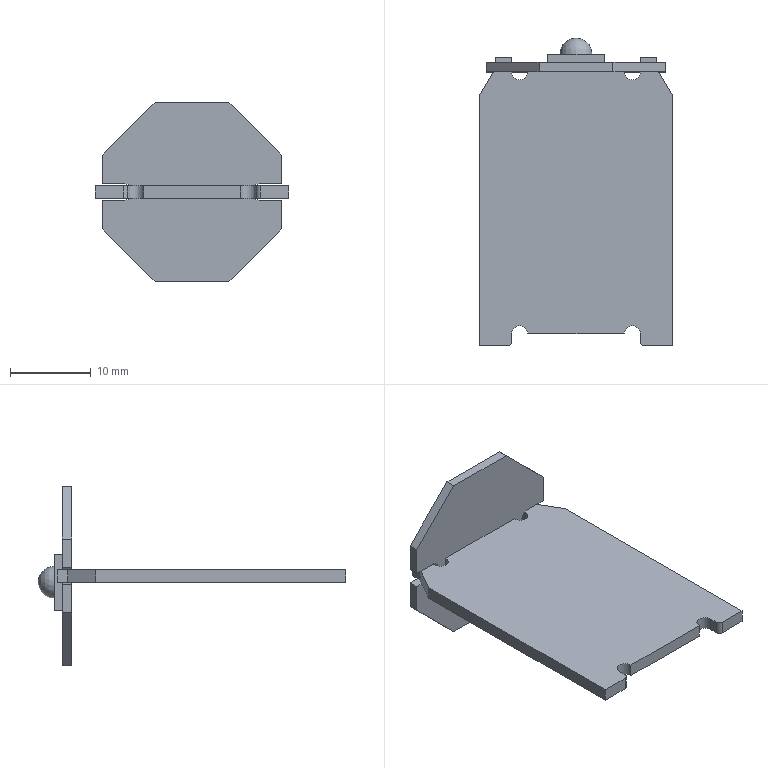Part | SolidWorks | features ICE 2, Extrusion 1, Revolution 1 | 3 solids | 49 faces | box 24 x 38.2 x 22.173 mm | volume 1798 mm3 | plane 40 | cylinder 8 | sphere 1 | commonest cylinder face diameters 2 x6 1 x2
STEP:
#1=CARTESIAN_POINT('',(-8.5,-17.9,0.));
#2=VERTEX_POINT('',#1);
#3=CARTESIAN_POINT('',(-8.,-17.4,0.));
#4=VERTEX_POINT('',#3);
#5=CARTESIAN_POINT('',(-8.5,-17.4,0.));
#6=DIRECTION('',(0.,0.,1.));
#7=DIRECTION('',(1.,0.,0.));
#8=AXIS2_PLACEMENT_3D('',#5,#6,#7);
#9=CIRCLE('',#8,0.5);
#10=EDGE_CURVE('',#2,#4,#9,.T.);
#11=ORIENTED_EDGE('',*,*,#10,.T.);
#12=CARTESIAN_POINT('',(-8.,-17.4,1.6));
#13=VERTEX_POINT('',#12);
#14=CARTESIAN_POINT('',(-8.,-17.4,1.6));
#15=DIRECTION('',(0.,0.,-1.));
#16=VECTOR('',#15,1000.);
#17=LINE('',#14,#16);
#18=EDGE_CURVE('',#13,#4,#17,.T.);
#19=ORIENTED_EDGE('',*,*,#18,.F.);
#20=CARTESIAN_POINT('',(-8.5,-17.9,1.6));
#21=VERTEX_POINT('',#20);
#22=CARTESIAN_POINT('',(-8.5,-17.4,1.6));
#23=DIRECTION('',(0.,0.,1.));
#24=DIRECTION('',(1.,0.,0.));
#25=AXIS2_PLACEMENT_3D('',#22,#23,#24);
#26=CIRCLE('',#25,0.5);
#27=EDGE_CURVE('',#21,#13,#26,.T.);
#28=ORIENTED_EDGE('',*,*,#27,.F.);
#29=CARTESIAN_POINT('',(-8.5,-17.9,1.6));
#30=DIRECTION('',(0.,0.,-1.));
#31=VECTOR('',#30,1000.);
#32=LINE('',#29,#31);
#33=EDGE_CURVE('',#21,#2,#32,.T.);
#34=ORIENTED_EDGE('',*,*,#33,.T.);
#35=EDGE_LOOP('',(#11,#19,#28,#34));
#36=FACE_OUTER_BOUND('',#35,.T.);
#37=CARTESIAN_POINT('',(-8.5,-17.4,1.6));
#38=DIRECTION('',(0.,0.,-1.));
#39=DIRECTION('',(-1.,0.,0.));
#40=AXIS2_PLACEMENT_3D('',#37,#38,#39);
#41=CYLINDRICAL_SURFACE('',#40,0.5);
#42=ADVANCED_FACE('',(#36),#41,.T.);
#43=CARTESIAN_POINT('',(-8.,-16.4,0.));
#44=VERTEX_POINT('',#43);
#45=CARTESIAN_POINT('',(-8.,-17.4,0.));
#46=DIRECTION('',(0.,1.,0.));
#47=VECTOR('',#46,1000.);
#48=LINE('',#45,#47);
#49=EDGE_CURVE('',#4,#44,#48,.T.);
#50=ORIENTED_EDGE('',*,*,#49,.T.);
#51=CARTESIAN_POINT('',(-8.,-16.4,1.6));
#52=VERTEX_POINT('',#51);
#53=CARTESIAN_POINT('',(-8.,-16.4,1.6));
#54=DIRECTION('',(0.,0.,-1.));
#55=VECTOR('',#54,1000.);
#56=LINE('',#53,#55);
#57=EDGE_CURVE('',#52,#44,#56,.T.);
#58=ORIENTED_EDGE('',*,*,#57,.F.);
#59=CARTESIAN_POINT('',(-8.,-17.4,1.6));
#60=DIRECTION('',(0.,1.,0.));
#61=VECTOR('',#60,1000.);
#62=LINE('',#59,#61);
#63=EDGE_CURVE('',#13,#52,#62,.T.);
#64=ORIENTED_EDGE('',*,*,#63,.F.);
#65=ORIENTED_EDGE('',*,*,#18,.T.);
#66=EDGE_LOOP('',(#50,#58,#64,#65));
#67=FACE_OUTER_BOUND('',#66,.T.);
#68=CARTESIAN_POINT('',(-8.,-17.4,1.6));
#69=DIRECTION('',(-1.,0.,0.));
#70=DIRECTION('',(0.,0.,1.));
#71=AXIS2_PLACEMENT_3D('',#68,#69,#70);
#72=PLANE('',#71);
#73=ADVANCED_FACE('',(#67),#72,.F.);
#74=CARTESIAN_POINT('',(-6.,-16.4,0.));
#75=VERTEX_POINT('',#74);
#76=CARTESIAN_POINT('',(-7.,-16.4,0.));
#77=DIRECTION('',(0.,0.,-1.));
#78=DIRECTION('',(1.,0.,0.));
#79=AXIS2_PLACEMENT_3D('',#76,#77,#78);
#80=CIRCLE('',#79,1.);
#81=EDGE_CURVE('',#44,#75,#80,.T.);
#82=ORIENTED_EDGE('',*,*,#81,.T.);
#83=CARTESIAN_POINT('',(-6.,-16.4,1.6));
#84=VERTEX_POINT('',#83);
#85=CARTESIAN_POINT('',(-6.,-16.4,1.6));
#86=DIRECTION('',(0.,0.,-1.));
#87=VECTOR('',#86,1000.);
#88=LINE('',#85,#87);
#89=EDGE_CURVE('',#84,#75,#88,.T.);
#90=ORIENTED_EDGE('',*,*,#89,.F.);
#91=CARTESIAN_POINT('',(-7.,-16.4,1.6));
#92=DIRECTION('',(0.,0.,-1.));
#93=DIRECTION('',(1.,0.,0.));
#94=AXIS2_PLACEMENT_3D('',#91,#92,#93);
#95=CIRCLE('',#94,1.);
#96=EDGE_CURVE('',#52,#84,#95,.T.);
#97=ORIENTED_EDGE('',*,*,#96,.F.);
#98=ORIENTED_EDGE('',*,*,#57,.T.);
#99=EDGE_LOOP('',(#82,#90,#97,#98));
#100=FACE_OUTER_BOUND('',#99,.T.);
#101=CARTESIAN_POINT('',(-7.,-16.4,1.6));
#102=DIRECTION('',(0.,0.,-1.));
#103=DIRECTION('',(-1.,0.,0.));
#104=AXIS2_PLACEMENT_3D('',#101,#102,#103);
#105=CYLINDRICAL_SURFACE('',#104,1.);
#106=ADVANCED_FACE('',(#100),#105,.F.);
#107=CARTESIAN_POINT('',(6.,-16.4,0.));
#108=VERTEX_POINT('',#107);
#109=CARTESIAN_POINT('',(-6.,-16.4,0.));
#110=DIRECTION('',(1.,0.,0.));
#111=VECTOR('',#110,1000.);
#112=LINE('',#109,#111);
#113=EDGE_CURVE('',#75,#108,#112,.T.);
#114=ORIENTED_EDGE('',*,*,#113,.T.);
#115=CARTESIAN_POINT('',(6.,-16.4,1.6));
#116=VERTEX_POINT('',#115);
#117=CARTESIAN_POINT('',(6.,-16.4,1.6));
#118=DIRECTION('',(0.,0.,-1.));
#119=VECTOR('',#118,1000.);
#120=LINE('',#117,#119);
#121=EDGE_CURVE('',#116,#108,#120,.T.);
#122=ORIENTED_EDGE('',*,*,#121,.F.);
#123=CARTESIAN_POINT('',(-6.,-16.4,1.6));
#124=DIRECTION('',(1.,0.,0.));
#125=VECTOR('',#124,1000.);
#126=LINE('',#123,#125);
#127=EDGE_CURVE('',#84,#116,#126,.T.);
#128=ORIENTED_EDGE('',*,*,#127,.F.);
#129=ORIENTED_EDGE('',*,*,#89,.T.);
#130=EDGE_LOOP('',(#114,#122,#128,#129));
#131=FACE_OUTER_BOUND('',#130,.T.);
#132=CARTESIAN_POINT('',(-6.,-16.4,1.6));
#133=DIRECTION('',(0.,1.,0.));
#134=DIRECTION('',(-1.,0.,0.));
#135=AXIS2_PLACEMENT_3D('',#132,#133,#134);
#136=PLANE('',#135);
#137=ADVANCED_FACE('',(#131),#136,.F.);
#138=CARTESIAN_POINT('',(8.,-16.4,0.));
#139=VERTEX_POINT('',#138);
#140=CARTESIAN_POINT('',(7.,-16.4,0.));
#141=DIRECTION('',(0.,0.,-1.));
#142=DIRECTION('',(1.,0.,0.));
#143=AXIS2_PLACEMENT_3D('',#140,#141,#142);
#144=CIRCLE('',#143,1.);
#145=EDGE_CURVE('',#108,#139,#144,.T.);
#146=ORIENTED_EDGE('',*,*,#145,.T.);
#147=CARTESIAN_POINT('',(8.,-16.4,1.6));
#148=VERTEX_POINT('',#147);
#149=CARTESIAN_POINT('',(8.,-16.4,1.6));
#150=DIRECTION('',(0.,0.,-1.));
#151=VECTOR('',#150,1000.);
#152=LINE('',#149,#151);
#153=EDGE_CURVE('',#148,#139,#152,.T.);
#154=ORIENTED_EDGE('',*,*,#153,.F.);
#155=CARTESIAN_POINT('',(7.,-16.4,1.6));
#156=DIRECTION('',(0.,0.,-1.));
#157=DIRECTION('',(1.,0.,0.));
#158=AXIS2_PLACEMENT_3D('',#155,#156,#157);
#159=CIRCLE('',#158,1.);
#160=EDGE_CURVE('',#116,#148,#159,.T.);
#161=ORIENTED_EDGE('',*,*,#160,.F.);
#162=ORIENTED_EDGE('',*,*,#121,.T.);
#163=EDGE_LOOP('',(#146,#154,#161,#162));
#164=FACE_OUTER_BOUND('',#163,.T.);
#165=CARTESIAN_POINT('',(7.,-16.4,1.6));
#166=DIRECTION('',(0.,0.,-1.));
#167=DIRECTION('',(-1.,0.,0.));
#168=AXIS2_PLACEMENT_3D('',#165,#166,#167);
#169=CYLINDRICAL_SURFACE('',#168,1.);
#170=ADVANCED_FACE('',(#164),#169,.F.);
#171=CARTESIAN_POINT('',(8.,-17.4,0.));
#172=VERTEX_POINT('',#171);
#173=CARTESIAN_POINT('',(8.,-16.4,0.));
#174=DIRECTION('',(0.,-1.,0.));
#175=VECTOR('',#174,1000.);
#176=LINE('',#173,#175);
#177=EDGE_CURVE('',#139,#172,#176,.T.);
#178=ORIENTED_EDGE('',*,*,#177,.T.);
#179=CARTESIAN_POINT('',(8.,-17.4,1.6));
#180=VERTEX_POINT('',#179);
#181=CARTESIAN_POINT('',(8.,-17.4,1.6));
#182=DIRECTION('',(0.,0.,-1.));
#183=VECTOR('',#182,1000.);
#184=LINE('',#181,#183);
#185=EDGE_CURVE('',#180,#172,#184,.T.);
#186=ORIENTED_EDGE('',*,*,#185,.F.);
#187=CARTESIAN_POINT('',(8.,-16.4,1.6));
#188=DIRECTION('',(0.,-1.,0.));
#189=VECTOR('',#188,1000.);
#190=LINE('',#187,#189);
#191=EDGE_CURVE('',#148,#180,#190,.T.);
#192=ORIENTED_EDGE('',*,*,#191,.F.);
#193=ORIENTED_EDGE('',*,*,#153,.T.);
#194=EDGE_LOOP('',(#178,#186,#192,#193));
#195=FACE_OUTER_BOUND('',#194,.T.);
#196=CARTESIAN_POINT('',(8.,-16.4,1.6));
#197=DIRECTION('',(1.,0.,0.));
#198=DIRECTION('',(0.,0.,-1.));
#199=AXIS2_PLACEMENT_3D('',#196,#197,#198);
#200=PLANE('',#199);
#201=ADVANCED_FACE('',(#195),#200,.F.);
#202=CARTESIAN_POINT('',(8.5,-17.9,0.));
#203=VERTEX_POINT('',#202);
#204=CARTESIAN_POINT('',(8.5,-17.4,0.));
#205=DIRECTION('',(0.,0.,1.));
#206=DIRECTION('',(1.,0.,0.));
#207=AXIS2_PLACEMENT_3D('',#204,#205,#206);
#208=CIRCLE('',#207,0.5);
#209=EDGE_CURVE('',#172,#203,#208,.T.);
#210=ORIENTED_EDGE('',*,*,#209,.T.);
#211=CARTESIAN_POINT('',(8.5,-17.9,1.6));
#212=VERTEX_POINT('',#211);
#213=CARTESIAN_POINT('',(8.5,-17.9,1.6));
#214=DIRECTION('',(0.,0.,-1.));
#215=VECTOR('',#214,1000.);
#216=LINE('',#213,#215);
#217=EDGE_CURVE('',#212,#203,#216,.T.);
#218=ORIENTED_EDGE('',*,*,#217,.F.);
#219=CARTESIAN_POINT('',(8.5,-17.4,1.6));
#220=DIRECTION('',(0.,0.,1.));
#221=DIRECTION('',(1.,0.,0.));
#222=AXIS2_PLACEMENT_3D('',#219,#220,#221);
#223=CIRCLE('',#222,0.5);
#224=EDGE_CURVE('',#180,#212,#223,.T.);
#225=ORIENTED_EDGE('',*,*,#224,.F.);
#226=ORIENTED_EDGE('',*,*,#185,.T.);
#227=EDGE_LOOP('',(#210,#218,#225,#226));
#228=FACE_OUTER_BOUND('',#227,.T.);
#229=CARTESIAN_POINT('',(8.5,-17.4,1.6));
#230=DIRECTION('',(0.,0.,-1.));
#231=DIRECTION('',(-1.,0.,0.));
#232=AXIS2_PLACEMENT_3D('',#229,#230,#231);
#233=CYLINDRICAL_SURFACE('',#232,0.5);
#234=ADVANCED_FACE('',(#228),#233,.T.);
#235=CARTESIAN_POINT('',(12.,-17.9,0.));
#236=VERTEX_POINT('',#235);
#237=CARTESIAN_POINT('',(8.5,-17.9,0.));
#238=DIRECTION('',(1.,0.,0.));
#239=VECTOR('',#238,1000.);
#240=LINE('',#237,#239);
#241=EDGE_CURVE('',#203,#236,#240,.T.);
#242=ORIENTED_EDGE('',*,*,#241,.T.);
#243=CARTESIAN_POINT('',(12.,-17.9,1.6));
#244=VERTEX_POINT('',#243);
#245=CARTESIAN_POINT('',(12.,-17.9,1.6));
#246=DIRECTION('',(0.,0.,-1.));
#247=VECTOR('',#246,1000.);
#248=LINE('',#245,#247);
#249=EDGE_CURVE('',#244,#236,#248,.T.);
#250=ORIENTED_EDGE('',*,*,#249,.F.);
#251=CARTESIAN_POINT('',(8.5,-17.9,1.6));
#252=DIRECTION('',(1.,0.,0.));
#253=VECTOR('',#252,1000.);
#254=LINE('',#251,#253);
#255=EDGE_CURVE('',#212,#244,#254,.T.);
#256=ORIENTED_EDGE('',*,*,#255,.F.);
#257=ORIENTED_EDGE('',*,*,#217,.T.);
#258=EDGE_LOOP('',(#242,#250,#256,#257));
#259=FACE_OUTER_BOUND('',#258,.T.);
#260=CARTESIAN_POINT('',(8.5,-17.9,1.6));
#261=DIRECTION('',(0.,1.,0.));
#262=DIRECTION('',(0.,0.,1.));
#263=AXIS2_PLACEMENT_3D('',#260,#261,#262);
#264=PLANE('',#263);
#265=ADVANCED_FACE('',(#259),#264,.F.);
#266=CARTESIAN_POINT('',(12.,13.136,0.));
#267=VERTEX_POINT('',#266);
#268=CARTESIAN_POINT('',(12.,-17.9,0.));
#269=DIRECTION('',(0.,1.,0.));
#270=VECTOR('',#269,1000.);
#271=LINE('',#268,#270);
#272=EDGE_CURVE('',#236,#267,#271,.T.);
#273=ORIENTED_EDGE('',*,*,#272,.T.);
#274=CARTESIAN_POINT('',(12.,13.136,1.6));
#275=VERTEX_POINT('',#274);
#276=CARTESIAN_POINT('',(12.,13.136,1.6));
#277=DIRECTION('',(0.,0.,-1.));
#278=VECTOR('',#277,1000.);
#279=LINE('',#276,#278);
#280=EDGE_CURVE('',#275,#267,#279,.T.);
#281=ORIENTED_EDGE('',*,*,#280,.F.);
#282=CARTESIAN_POINT('',(12.,-17.9,1.6));
#283=DIRECTION('',(0.,1.,0.));
#284=VECTOR('',#283,1000.);
#285=LINE('',#282,#284);
#286=EDGE_CURVE('',#244,#275,#285,.T.);
#287=ORIENTED_EDGE('',*,*,#286,.F.);
#288=ORIENTED_EDGE('',*,*,#249,.T.);
#289=EDGE_LOOP('',(#273,#281,#287,#288));
#290=FACE_OUTER_BOUND('',#289,.T.);
#291=CARTESIAN_POINT('',(12.,-17.9,1.6));
#292=DIRECTION('',(-1.,0.,0.));
#293=DIRECTION('',(0.,0.,1.));
#294=AXIS2_PLACEMENT_3D('',#291,#292,#293);
#295=PLANE('',#294);
#296=ADVANCED_FACE('',(#290),#295,.F.);
#297=CARTESIAN_POINT('',(10.,16.6,0.));
#298=VERTEX_POINT('',#297);
#299=CARTESIAN_POINT('',(12.,13.136,0.));
#300=DIRECTION('',(-0.5,0.866,0.));
#301=VECTOR('',#300,1000.);
#302=LINE('',#299,#301);
#303=EDGE_CURVE('',#267,#298,#302,.T.);
#304=ORIENTED_EDGE('',*,*,#303,.T.);
#305=CARTESIAN_POINT('',(10.,16.6,1.6));
#306=VERTEX_POINT('',#305);
#307=CARTESIAN_POINT('',(10.,16.6,1.6));
#308=DIRECTION('',(0.,0.,-1.));
#309=VECTOR('',#308,1000.);
#310=LINE('',#307,#309);
#311=EDGE_CURVE('',#306,#298,#310,.T.);
#312=ORIENTED_EDGE('',*,*,#311,.F.);
#313=CARTESIAN_POINT('',(12.,13.136,1.6));
#314=DIRECTION('',(-0.5,0.866,0.));
#315=VECTOR('',#314,1000.);
#316=LINE('',#313,#315);
#317=EDGE_CURVE('',#275,#306,#316,.T.);
#318=ORIENTED_EDGE('',*,*,#317,.F.);
#319=ORIENTED_EDGE('',*,*,#280,.T.);
#320=EDGE_LOOP('',(#304,#312,#318,#319));
#321=FACE_OUTER_BOUND('',#320,.T.);
#322=CARTESIAN_POINT('',(12.,13.136,1.6));
#323=DIRECTION('',(-0.866,-0.5,0.));
#324=DIRECTION('',(0.5,-0.866,0.));
#325=AXIS2_PLACEMENT_3D('',#322,#323,#324);
#326=PLANE('',#325);
#327=ADVANCED_FACE('',(#321),#326,.F.);
#328=CARTESIAN_POINT('',(10.,17.9,0.));
#329=VERTEX_POINT('',#328);
#330=CARTESIAN_POINT('',(10.,16.6,0.));
#331=DIRECTION('',(0.,1.,0.));
#332=VECTOR('',#331,1000.);
#333=LINE('',#330,#332);
#334=EDGE_CURVE('',#298,#329,#333,.T.);
#335=ORIENTED_EDGE('',*,*,#334,.T.);
#336=CARTESIAN_POINT('',(10.,17.9,1.6));
#337=VERTEX_POINT('',#336);
#338=CARTESIAN_POINT('',(10.,17.9,1.6));
#339=DIRECTION('',(0.,0.,-1.));
#340=VECTOR('',#339,1000.);
#341=LINE('',#338,#340);
#342=EDGE_CURVE('',#337,#329,#341,.T.);
#343=ORIENTED_EDGE('',*,*,#342,.F.);
#344=CARTESIAN_POINT('',(10.,16.6,1.6));
#345=DIRECTION('',(0.,1.,0.));
#346=VECTOR('',#345,1000.);
#347=LINE('',#344,#346);
#348=EDGE_CURVE('',#306,#337,#347,.T.);
#349=ORIENTED_EDGE('',*,*,#348,.F.);
#350=ORIENTED_EDGE('',*,*,#311,.T.);
#351=EDGE_LOOP('',(#335,#343,#349,#350));
#352=FACE_OUTER_BOUND('',#351,.T.);
#353=CARTESIAN_POINT('',(10.,16.6,1.6));
#354=DIRECTION('',(-1.,0.,0.));
#355=DIRECTION('',(0.,0.,1.));
#356=AXIS2_PLACEMENT_3D('',#353,#354,#355);
#357=PLANE('',#356);
#358=ADVANCED_FACE('',(#352),#357,.F.);
#359=CARTESIAN_POINT('',(8.,17.9,0.));
#360=VERTEX_POINT('',#359);
#361=CARTESIAN_POINT('',(10.,17.9,0.));
#362=DIRECTION('',(-1.,0.,0.));
#363=VECTOR('',#362,1000.);
#364=LINE('',#361,#363);
#365=EDGE_CURVE('',#329,#360,#364,.T.);
#366=ORIENTED_EDGE('',*,*,#365,.T.);
#367=CARTESIAN_POINT('',(8.,17.9,1.6));
#368=VERTEX_POINT('',#367);
#369=CARTESIAN_POINT('',(8.,17.9,1.6));
#370=DIRECTION('',(0.,0.,-1.));
#371=VECTOR('',#370,1000.);
#372=LINE('',#369,#371);
#373=EDGE_CURVE('',#368,#360,#372,.T.);
#374=ORIENTED_EDGE('',*,*,#373,.F.);
#375=CARTESIAN_POINT('',(10.,17.9,1.6));
#376=DIRECTION('',(-1.,0.,0.));
#377=VECTOR('',#376,1000.);
#378=LINE('',#375,#377);
#379=EDGE_CURVE('',#337,#368,#378,.T.);
#380=ORIENTED_EDGE('',*,*,#379,.F.);
#381=ORIENTED_EDGE('',*,*,#342,.T.);
#382=EDGE_LOOP('',(#366,#374,#380,#381));
#383=FACE_OUTER_BOUND('',#382,.T.);
#384=CARTESIAN_POINT('',(10.,17.9,1.6));
#385=DIRECTION('',(0.,-1.,0.));
#386=DIRECTION('',(0.,0.,-1.));
#387=AXIS2_PLACEMENT_3D('',#384,#385,#386);
#388=PLANE('',#387);
#389=ADVANCED_FACE('',(#383),#388,.F.);
#390=CARTESIAN_POINT('',(8.,16.1,0.));
#391=VERTEX_POINT('',#390);
#392=CARTESIAN_POINT('',(8.,17.9,0.));
#393=DIRECTION('',(0.,-1.,0.));
#394=VECTOR('',#393,1000.);
#395=LINE('',#392,#394);
#396=EDGE_CURVE('',#360,#391,#395,.T.);
#397=ORIENTED_EDGE('',*,*,#396,.T.);
#398=CARTESIAN_POINT('',(8.,16.1,1.6));
#399=VERTEX_POINT('',#398);
#400=CARTESIAN_POINT('',(8.,16.1,1.6));
#401=DIRECTION('',(0.,0.,-1.));
#402=VECTOR('',#401,1000.);
#403=LINE('',#400,#402);
#404=EDGE_CURVE('',#399,#391,#403,.T.);
#405=ORIENTED_EDGE('',*,*,#404,.F.);
#406=CARTESIAN_POINT('',(8.,17.9,1.6));
#407=DIRECTION('',(0.,-1.,0.));
#408=VECTOR('',#407,1000.);
#409=LINE('',#406,#408);
#410=EDGE_CURVE('',#368,#399,#409,.T.);
#411=ORIENTED_EDGE('',*,*,#410,.F.);
#412=ORIENTED_EDGE('',*,*,#373,.T.);
#413=EDGE_LOOP('',(#397,#405,#411,#412));
#414=FACE_OUTER_BOUND('',#413,.T.);
#415=CARTESIAN_POINT('',(8.,17.9,1.6));
#416=DIRECTION('',(1.,0.,0.));
#417=DIRECTION('',(0.,0.,-1.));
#418=AXIS2_PLACEMENT_3D('',#415,#416,#417);
#419=PLANE('',#418);
#420=ADVANCED_FACE('',(#414),#419,.F.);
#421=CARTESIAN_POINT('',(6.,16.1,0.));
#422=VERTEX_POINT('',#421);
#423=CARTESIAN_POINT('',(7.,16.1,0.));
#424=DIRECTION('',(0.,0.,-1.));
#425=DIRECTION('',(1.,0.,0.));
#426=AXIS2_PLACEMENT_3D('',#423,#424,#425);
#427=CIRCLE('',#426,1.);
#428=EDGE_CURVE('',#391,#422,#427,.T.);
#429=ORIENTED_EDGE('',*,*,#428,.T.);
#430=CARTESIAN_POINT('',(6.,16.1,1.6));
#431=VERTEX_POINT('',#430);
#432=CARTESIAN_POINT('',(6.,16.1,1.6));
#433=DIRECTION('',(0.,0.,-1.));
#434=VECTOR('',#433,1000.);
#435=LINE('',#432,#434);
#436=EDGE_CURVE('',#431,#422,#435,.T.);
#437=ORIENTED_EDGE('',*,*,#436,.F.);
#438=CARTESIAN_POINT('',(7.,16.1,1.6));
#439=DIRECTION('',(0.,0.,-1.));
#440=DIRECTION('',(1.,0.,0.));
#441=AXIS2_PLACEMENT_3D('',#438,#439,#440);
#442=CIRCLE('',#441,1.);
#443=EDGE_CURVE('',#399,#431,#442,.T.);
#444=ORIENTED_EDGE('',*,*,#443,.F.);
#445=ORIENTED_EDGE('',*,*,#404,.T.);
#446=EDGE_LOOP('',(#429,#437,#444,#445));
#447=FACE_OUTER_BOUND('',#446,.T.);
#448=CARTESIAN_POINT('',(7.,16.1,1.6));
#449=DIRECTION('',(0.,0.,-1.));
#450=DIRECTION('',(-1.,0.,0.));
#451=AXIS2_PLACEMENT_3D('',#448,#449,#450);
#452=CYLINDRICAL_SURFACE('',#451,1.);
#453=ADVANCED_FACE('',(#447),#452,.F.);
#454=CARTESIAN_POINT('',(-6.,16.1,0.));
#455=VERTEX_POINT('',#454);
#456=CARTESIAN_POINT('',(6.,16.1,0.));
#457=DIRECTION('',(-1.,0.,0.));
#458=VECTOR('',#457,1000.);
#459=LINE('',#456,#458);
#460=EDGE_CURVE('',#422,#455,#459,.T.);
#461=ORIENTED_EDGE('',*,*,#460,.T.);
#462=CARTESIAN_POINT('',(-6.,16.1,1.6));
#463=VERTEX_POINT('',#462);
#464=CARTESIAN_POINT('',(-6.,16.1,1.6));
#465=DIRECTION('',(0.,0.,-1.));
#466=VECTOR('',#465,1000.);
#467=LINE('',#464,#466);
#468=EDGE_CURVE('',#463,#455,#467,.T.);
#469=ORIENTED_EDGE('',*,*,#468,.F.);
#470=CARTESIAN_POINT('',(6.,16.1,1.6));
#471=DIRECTION('',(-1.,0.,0.));
#472=VECTOR('',#471,1000.);
#473=LINE('',#470,#472);
#474=EDGE_CURVE('',#431,#463,#473,.T.);
#475=ORIENTED_EDGE('',*,*,#474,.F.);
#476=ORIENTED_EDGE('',*,*,#436,.T.);
#477=EDGE_LOOP('',(#461,#469,#475,#476));
#478=FACE_OUTER_BOUND('',#477,.T.);
#479=CARTESIAN_POINT('',(6.,16.1,1.6));
#480=DIRECTION('',(0.,-1.,0.));
#481=DIRECTION('',(0.,0.,-1.));
#482=AXIS2_PLACEMENT_3D('',#479,#480,#481);
#483=PLANE('',#482);
#484=ADVANCED_FACE('',(#478),#483,.F.);
#485=CARTESIAN_POINT('',(-8.,16.1,0.));
#486=VERTEX_POINT('',#485);
#487=CARTESIAN_POINT('',(-7.,16.1,0.));
#488=DIRECTION('',(0.,0.,-1.));
#489=DIRECTION('',(1.,0.,0.));
#490=AXIS2_PLACEMENT_3D('',#487,#488,#489);
#491=CIRCLE('',#490,1.);
#492=EDGE_CURVE('',#455,#486,#491,.T.);
#493=ORIENTED_EDGE('',*,*,#492,.T.);
#494=CARTESIAN_POINT('',(-8.,16.1,1.6));
#495=VERTEX_POINT('',#494);
#496=CARTESIAN_POINT('',(-8.,16.1,1.6));
#497=DIRECTION('',(0.,0.,-1.));
#498=VECTOR('',#497,1000.);
#499=LINE('',#496,#498);
#500=EDGE_CURVE('',#495,#486,#499,.T.);
#501=ORIENTED_EDGE('',*,*,#500,.F.);
#502=CARTESIAN_POINT('',(-7.,16.1,1.6));
#503=DIRECTION('',(0.,0.,-1.));
#504=DIRECTION('',(1.,0.,0.));
#505=AXIS2_PLACEMENT_3D('',#502,#503,#504);
#506=CIRCLE('',#505,1.);
#507=EDGE_CURVE('',#463,#495,#506,.T.);
#508=ORIENTED_EDGE('',*,*,#507,.F.);
#509=ORIENTED_EDGE('',*,*,#468,.T.);
#510=EDGE_LOOP('',(#493,#501,#508,#509));
#511=FACE_OUTER_BOUND('',#510,.T.);
#512=CARTESIAN_POINT('',(-7.,16.1,1.6));
#513=DIRECTION('',(0.,0.,-1.));
#514=DIRECTION('',(-1.,0.,0.));
#515=AXIS2_PLACEMENT_3D('',#512,#513,#514);
#516=CYLINDRICAL_SURFACE('',#515,1.);
#517=ADVANCED_FACE('',(#511),#516,.F.);
#518=CARTESIAN_POINT('',(-8.,17.9,0.));
#519=VERTEX_POINT('',#518);
#520=CARTESIAN_POINT('',(-8.,16.1,0.));
#521=DIRECTION('',(0.,1.,0.));
#522=VECTOR('',#521,1000.);
#523=LINE('',#520,#522);
#524=EDGE_CURVE('',#486,#519,#523,.T.);
#525=ORIENTED_EDGE('',*,*,#524,.T.);
#526=CARTESIAN_POINT('',(-8.,17.9,1.6));
#527=VERTEX_POINT('',#526);
#528=CARTESIAN_POINT('',(-8.,17.9,1.6));
#529=DIRECTION('',(0.,0.,-1.));
#530=VECTOR('',#529,1000.);
#531=LINE('',#528,#530);
#532=EDGE_CURVE('',#527,#519,#531,.T.);
#533=ORIENTED_EDGE('',*,*,#532,.F.);
#534=CARTESIAN_POINT('',(-8.,16.1,1.6));
#535=DIRECTION('',(0.,1.,0.));
#536=VECTOR('',#535,1000.);
#537=LINE('',#534,#536);
#538=EDGE_CURVE('',#495,#527,#537,.T.);
#539=ORIENTED_EDGE('',*,*,#538,.F.);
#540=ORIENTED_EDGE('',*,*,#500,.T.);
#541=EDGE_LOOP('',(#525,#533,#539,#540));
#542=FACE_OUTER_BOUND('',#541,.T.);
#543=CARTESIAN_POINT('',(-8.,16.1,1.6));
#544=DIRECTION('',(-1.,0.,0.));
#545=DIRECTION('',(0.,0.,1.));
#546=AXIS2_PLACEMENT_3D('',#543,#544,#545);
#547=PLANE('',#546);
#548=ADVANCED_FACE('',(#542),#547,.F.);
#549=CARTESIAN_POINT('',(-10.,17.9,0.));
#550=VERTEX_POINT('',#549);
#551=CARTESIAN_POINT('',(-8.,17.9,0.));
#552=DIRECTION('',(-1.,0.,0.));
#553=VECTOR('',#552,1000.);
#554=LINE('',#551,#553);
#555=EDGE_CURVE('',#519,#550,#554,.T.);
#556=ORIENTED_EDGE('',*,*,#555,.T.);
#557=CARTESIAN_POINT('',(-10.,17.9,1.6));
#558=VERTEX_POINT('',#557);
#559=CARTESIAN_POINT('',(-10.,17.9,1.6));
#560=DIRECTION('',(0.,0.,-1.));
#561=VECTOR('',#560,1000.);
#562=LINE('',#559,#561);
#563=EDGE_CURVE('',#558,#550,#562,.T.);
#564=ORIENTED_EDGE('',*,*,#563,.F.);
#565=CARTESIAN_POINT('',(-8.,17.9,1.6));
#566=DIRECTION('',(-1.,0.,0.));
#567=VECTOR('',#566,1000.);
#568=LINE('',#565,#567);
#569=EDGE_CURVE('',#527,#558,#568,.T.);
#570=ORIENTED_EDGE('',*,*,#569,.F.);
#571=ORIENTED_EDGE('',*,*,#532,.T.);
#572=EDGE_LOOP('',(#556,#564,#570,#571));
#573=FACE_OUTER_BOUND('',#572,.T.);
#574=CARTESIAN_POINT('',(-8.,17.9,1.6));
#575=DIRECTION('',(0.,-1.,0.));
#576=DIRECTION('',(0.,0.,-1.));
#577=AXIS2_PLACEMENT_3D('',#574,#575,#576);
#578=PLANE('',#577);
#579=ADVANCED_FACE('',(#573),#578,.F.);
#580=CARTESIAN_POINT('',(-10.,16.6,0.));
#581=VERTEX_POINT('',#580);
#582=CARTESIAN_POINT('',(-10.,17.9,0.));
#583=DIRECTION('',(0.,-1.,0.));
#584=VECTOR('',#583,1000.);
#585=LINE('',#582,#584);
#586=EDGE_CURVE('',#550,#581,#585,.T.);
#587=ORIENTED_EDGE('',*,*,#586,.T.);
#588=CARTESIAN_POINT('',(-10.,16.6,1.6));
#589=VERTEX_POINT('',#588);
#590=CARTESIAN_POINT('',(-10.,16.6,1.6));
#591=DIRECTION('',(0.,0.,-1.));
#592=VECTOR('',#591,1000.);
#593=LINE('',#590,#592);
#594=EDGE_CURVE('',#589,#581,#593,.T.);
#595=ORIENTED_EDGE('',*,*,#594,.F.);
#596=CARTESIAN_POINT('',(-10.,17.9,1.6));
#597=DIRECTION('',(0.,-1.,0.));
#598=VECTOR('',#597,1000.);
#599=LINE('',#596,#598);
#600=EDGE_CURVE('',#558,#589,#599,.T.);
#601=ORIENTED_EDGE('',*,*,#600,.F.);
#602=ORIENTED_EDGE('',*,*,#563,.T.);
#603=EDGE_LOOP('',(#587,#595,#601,#602));
#604=FACE_OUTER_BOUND('',#603,.T.);
#605=CARTESIAN_POINT('',(-10.,17.9,1.6));
#606=DIRECTION('',(1.,0.,0.));
#607=DIRECTION('',(0.,0.,-1.));
#608=AXIS2_PLACEMENT_3D('',#605,#606,#607);
#609=PLANE('',#608);
#610=ADVANCED_FACE('',(#604),#609,.F.);
#611=CARTESIAN_POINT('',(-12.,13.136,0.));
#612=VERTEX_POINT('',#611);
#613=CARTESIAN_POINT('',(-10.,16.6,0.));
#614=DIRECTION('',(-0.5,-0.866,0.));
#615=VECTOR('',#614,1000.);
#616=LINE('',#613,#615);
#617=EDGE_CURVE('',#581,#612,#616,.T.);
#618=ORIENTED_EDGE('',*,*,#617,.T.);
#619=CARTESIAN_POINT('',(-12.,13.136,1.6));
#620=VERTEX_POINT('',#619);
#621=CARTESIAN_POINT('',(-12.,13.136,1.6));
#622=DIRECTION('',(0.,0.,-1.));
#623=VECTOR('',#622,1000.);
#624=LINE('',#621,#623);
#625=EDGE_CURVE('',#620,#612,#624,.T.);
#626=ORIENTED_EDGE('',*,*,#625,.F.);
#627=CARTESIAN_POINT('',(-10.,16.6,1.6));
#628=DIRECTION('',(-0.5,-0.866,0.));
#629=VECTOR('',#628,1000.);
#630=LINE('',#627,#629);
#631=EDGE_CURVE('',#589,#620,#630,.T.);
#632=ORIENTED_EDGE('',*,*,#631,.F.);
#633=ORIENTED_EDGE('',*,*,#594,.T.);
#634=EDGE_LOOP('',(#618,#626,#632,#633));
#635=FACE_OUTER_BOUND('',#634,.T.);
#636=CARTESIAN_POINT('',(-10.,16.6,1.6));
#637=DIRECTION('',(0.866,-0.5,0.));
#638=DIRECTION('',(0.5,0.866,0.));
#639=AXIS2_PLACEMENT_3D('',#636,#637,#638);
#640=PLANE('',#639);
#641=ADVANCED_FACE('',(#635),#640,.F.);
#642=CARTESIAN_POINT('',(-12.,-17.9,0.));
#643=VERTEX_POINT('',#642);
#644=CARTESIAN_POINT('',(-12.,13.136,0.));
#645=DIRECTION('',(0.,-1.,0.));
#646=VECTOR('',#645,1000.);
#647=LINE('',#644,#646);
#648=EDGE_CURVE('',#612,#643,#647,.T.);
#649=ORIENTED_EDGE('',*,*,#648,.T.);
#650=CARTESIAN_POINT('',(-12.,-17.9,1.6));
#651=VERTEX_POINT('',#650);
#652=CARTESIAN_POINT('',(-12.,-17.9,1.6));
#653=DIRECTION('',(0.,0.,-1.));
#654=VECTOR('',#653,1000.);
#655=LINE('',#652,#654);
#656=EDGE_CURVE('',#651,#643,#655,.T.);
#657=ORIENTED_EDGE('',*,*,#656,.F.);
#658=CARTESIAN_POINT('',(-12.,13.136,1.6));
#659=DIRECTION('',(0.,-1.,0.));
#660=VECTOR('',#659,1000.);
#661=LINE('',#658,#660);
#662=EDGE_CURVE('',#620,#651,#661,.T.);
#663=ORIENTED_EDGE('',*,*,#662,.F.);
#664=ORIENTED_EDGE('',*,*,#625,.T.);
#665=EDGE_LOOP('',(#649,#657,#663,#664));
#666=FACE_OUTER_BOUND('',#665,.T.);
#667=CARTESIAN_POINT('',(-12.,13.136,1.6));
#668=DIRECTION('',(1.,0.,0.));
#669=DIRECTION('',(0.,0.,-1.));
#670=AXIS2_PLACEMENT_3D('',#667,#668,#669);
#671=PLANE('',#670);
#672=ADVANCED_FACE('',(#666),#671,.F.);
#673=CARTESIAN_POINT('',(-12.,-17.9,0.));
#674=DIRECTION('',(1.,0.,0.));
#675=VECTOR('',#674,1000.);
#676=LINE('',#673,#675);
#677=EDGE_CURVE('',#643,#2,#676,.T.);
#678=ORIENTED_EDGE('',*,*,#677,.T.);
#679=ORIENTED_EDGE('',*,*,#33,.F.);
#680=CARTESIAN_POINT('',(-12.,-17.9,1.6));
#681=DIRECTION('',(1.,0.,0.));
#682=VECTOR('',#681,1000.);
#683=LINE('',#680,#682);
#684=EDGE_CURVE('',#651,#21,#683,.T.);
#685=ORIENTED_EDGE('',*,*,#684,.F.);
#686=ORIENTED_EDGE('',*,*,#656,.T.);
#687=EDGE_LOOP('',(#678,#679,#685,#686));
#688=FACE_OUTER_BOUND('',#687,.T.);
#689=CARTESIAN_POINT('',(-12.,-17.9,1.6));
#690=DIRECTION('',(0.,1.,0.));
#691=DIRECTION('',(0.,0.,1.));
#692=AXIS2_PLACEMENT_3D('',#689,#690,#691);
#693=PLANE('',#692);
#694=ADVANCED_FACE('',(#688),#693,.F.);
#695=ORIENTED_EDGE('',*,*,#27,.T.);
#696=ORIENTED_EDGE('',*,*,#63,.T.);
#697=ORIENTED_EDGE('',*,*,#96,.T.);
#698=ORIENTED_EDGE('',*,*,#127,.T.);
#699=ORIENTED_EDGE('',*,*,#160,.T.);
#700=ORIENTED_EDGE('',*,*,#191,.T.);
#701=ORIENTED_EDGE('',*,*,#224,.T.);
#702=ORIENTED_EDGE('',*,*,#255,.T.);
#703=ORIENTED_EDGE('',*,*,#286,.T.);
#704=ORIENTED_EDGE('',*,*,#317,.T.);
#705=ORIENTED_EDGE('',*,*,#348,.T.);
#706=ORIENTED_EDGE('',*,*,#379,.T.);
#707=ORIENTED_EDGE('',*,*,#410,.T.);
#708=ORIENTED_EDGE('',*,*,#443,.T.);
#709=ORIENTED_EDGE('',*,*,#474,.T.);
#710=ORIENTED_EDGE('',*,*,#507,.T.);
#711=ORIENTED_EDGE('',*,*,#538,.T.);
#712=ORIENTED_EDGE('',*,*,#569,.T.);
#713=ORIENTED_EDGE('',*,*,#600,.T.);
#714=ORIENTED_EDGE('',*,*,#631,.T.);
#715=ORIENTED_EDGE('',*,*,#662,.T.);
#716=ORIENTED_EDGE('',*,*,#684,.T.);
#717=EDGE_LOOP('',(#695,#696,#697,#698,#699,#700,#701,#702,#703,#704,#705,#706,#707,#708,#709,#710,#711,#712,#713,#714,#715,#716));
#718=FACE_OUTER_BOUND('',#717,.T.);
#719=CARTESIAN_POINT('',(-8.5,-17.4,1.6));
#720=DIRECTION('',(0.,0.,1.));
#721=DIRECTION('',(1.,0.,0.));
#722=AXIS2_PLACEMENT_3D('',#719,#720,#721);
#723=PLANE('',#722);
#724=ADVANCED_FACE('',(#718),#723,.T.);
#725=ORIENTED_EDGE('',*,*,#10,.F.);
#726=ORIENTED_EDGE('',*,*,#677,.F.);
#727=ORIENTED_EDGE('',*,*,#648,.F.);
#728=ORIENTED_EDGE('',*,*,#617,.F.);
#729=ORIENTED_EDGE('',*,*,#586,.F.);
#730=ORIENTED_EDGE('',*,*,#555,.F.);
#731=ORIENTED_EDGE('',*,*,#524,.F.);
#732=ORIENTED_EDGE('',*,*,#492,.F.);
#733=ORIENTED_EDGE('',*,*,#460,.F.);
#734=ORIENTED_EDGE('',*,*,#428,.F.);
#735=ORIENTED_EDGE('',*,*,#396,.F.);
#736=ORIENTED_EDGE('',*,*,#365,.F.);
#737=ORIENTED_EDGE('',*,*,#334,.F.);
#738=ORIENTED_EDGE('',*,*,#303,.F.);
#739=ORIENTED_EDGE('',*,*,#272,.F.);
#740=ORIENTED_EDGE('',*,*,#241,.F.);
#741=ORIENTED_EDGE('',*,*,#209,.F.);
#742=ORIENTED_EDGE('',*,*,#177,.F.);
#743=ORIENTED_EDGE('',*,*,#145,.F.);
#744=ORIENTED_EDGE('',*,*,#113,.F.);
#745=ORIENTED_EDGE('',*,*,#81,.F.);
#746=ORIENTED_EDGE('',*,*,#49,.F.);
#747=EDGE_LOOP('',(#725,#726,#727,#728,#729,#730,#731,#732,#733,#734,#735,#736,#737,#738,#739,#740,#741,#742,#743,#744,#745,#746));
#748=FACE_OUTER_BOUND('',#747,.T.);
#749=CARTESIAN_POINT('',(-8.5,-17.4,0.));
#750=DIRECTION('',(0.,0.,1.));
#751=DIRECTION('',(1.,0.,0.));
#752=AXIS2_PLACEMENT_3D('',#749,#750,#751);
#753=PLANE('',#752);
#754=ADVANCED_FACE('',(#748),#753,.F.);
#755=CLOSED_SHELL('',(#42,#73,#106,#137,#170,#201,#234,#265,#296,#327,#358,#389,#420,#453,#484,#517,#548,#579,#610,#641,#672,#694,#724,#754));
#756=MANIFOLD_SOLID_BREP('',#755);
#757=CARTESIAN_POINT('',(-8.337,16.1,1.8));
#758=VERTEX_POINT('',#757);
#759=CARTESIAN_POINT('',(-11.087,16.1,1.8));
#760=VERTEX_POINT('',#759);
#761=CARTESIAN_POINT('',(-8.337,16.1,1.8));
#762=DIRECTION('',(-1.,0.,0.));
#763=VECTOR('',#762,1000.);
#764=LINE('',#761,#763);
#765=EDGE_CURVE('',#758,#760,#764,.T.);
#766=ORIENTED_EDGE('',*,*,#765,.T.);
#767=CARTESIAN_POINT('',(-11.087,17.3,1.8));
#768=VERTEX_POINT('',#767);
#769=CARTESIAN_POINT('',(-11.087,17.3,1.8));
#770=DIRECTION('',(0.,-1.,0.));
#771=VECTOR('',#770,1000.);
#772=LINE('',#769,#771);
#773=EDGE_CURVE('',#768,#760,#772,.T.);
#774=ORIENTED_EDGE('',*,*,#773,.F.);
#775=CARTESIAN_POINT('',(-8.337,17.3,1.8));
#776=VERTEX_POINT('',#775);
#777=CARTESIAN_POINT('',(-8.337,17.3,1.8));
#778=DIRECTION('',(-1.,0.,0.));
#779=VECTOR('',#778,1000.);
#780=LINE('',#777,#779);
#781=EDGE_CURVE('',#776,#768,#780,.T.);
#782=ORIENTED_EDGE('',*,*,#781,.F.);
#783=CARTESIAN_POINT('',(-8.337,17.3,1.8));
#784=DIRECTION('',(0.,-1.,0.));
#785=VECTOR('',#784,1000.);
#786=LINE('',#783,#785);
#787=EDGE_CURVE('',#776,#758,#786,.T.);
#788=ORIENTED_EDGE('',*,*,#787,.T.);
#789=EDGE_LOOP('',(#766,#774,#782,#788));
#790=FACE_OUTER_BOUND('',#789,.T.);
#791=CARTESIAN_POINT('',(-8.337,17.3,1.8));
#792=DIRECTION('',(0.,0.,1.));
#793=DIRECTION('',(1.,0.,0.));
#794=AXIS2_PLACEMENT_3D('',#791,#792,#793);
#795=PLANE('',#794);
#796=ADVANCED_FACE('',(#790),#795,.F.);
#797=CARTESIAN_POINT('',(-11.087,16.1,5.392));
#798=VERTEX_POINT('',#797);
#799=CARTESIAN_POINT('',(-11.087,16.1,1.8));
#800=DIRECTION('',(0.,0.,1.));
#801=VECTOR('',#800,1000.);
#802=LINE('',#799,#801);
#803=EDGE_CURVE('',#760,#798,#802,.T.);
#804=ORIENTED_EDGE('',*,*,#803,.T.);
#805=CARTESIAN_POINT('',(-11.087,17.3,5.392));
#806=VERTEX_POINT('',#805);
#807=CARTESIAN_POINT('',(-11.087,17.3,5.392));
#808=DIRECTION('',(0.,-1.,0.));
#809=VECTOR('',#808,1000.);
#810=LINE('',#807,#809);
#811=EDGE_CURVE('',#806,#798,#810,.T.);
#812=ORIENTED_EDGE('',*,*,#811,.F.);
#813=CARTESIAN_POINT('',(-11.087,17.3,1.8));
#814=DIRECTION('',(0.,0.,1.));
#815=VECTOR('',#814,1000.);
#816=LINE('',#813,#815);
#817=EDGE_CURVE('',#768,#806,#816,.T.);
#818=ORIENTED_EDGE('',*,*,#817,.F.);
#819=ORIENTED_EDGE('',*,*,#773,.T.);
#820=EDGE_LOOP('',(#804,#812,#818,#819));
#821=FACE_OUTER_BOUND('',#820,.T.);
#822=CARTESIAN_POINT('',(-11.087,17.3,1.8));
#823=DIRECTION('',(1.,0.,0.));
#824=DIRECTION('',(0.,0.,-1.));
#825=AXIS2_PLACEMENT_3D('',#822,#823,#824);
#826=PLANE('',#825);
#827=ADVANCED_FACE('',(#821),#826,.F.);
#828=CARTESIAN_POINT('',(-4.592,16.1,11.887));
#829=VERTEX_POINT('',#828);
#830=CARTESIAN_POINT('',(-11.087,16.1,5.392));
#831=DIRECTION('',(0.7071,0.,0.7071));
#832=VECTOR('',#831,1000.);
#833=LINE('',#830,#832);
#834=EDGE_CURVE('',#798,#829,#833,.T.);
#835=ORIENTED_EDGE('',*,*,#834,.T.);
#836=CARTESIAN_POINT('',(-4.592,17.3,11.887));
#837=VERTEX_POINT('',#836);
#838=CARTESIAN_POINT('',(-4.592,17.3,11.887));
#839=DIRECTION('',(0.,-1.,0.));
#840=VECTOR('',#839,1000.);
#841=LINE('',#838,#840);
#842=EDGE_CURVE('',#837,#829,#841,.T.);
#843=ORIENTED_EDGE('',*,*,#842,.F.);
#844=CARTESIAN_POINT('',(-11.087,17.3,5.392));
#845=DIRECTION('',(0.7071,0.,0.7071));
#846=VECTOR('',#845,1000.);
#847=LINE('',#844,#846);
#848=EDGE_CURVE('',#806,#837,#847,.T.);
#849=ORIENTED_EDGE('',*,*,#848,.F.);
#850=ORIENTED_EDGE('',*,*,#811,.T.);
#851=EDGE_LOOP('',(#835,#843,#849,#850));
#852=FACE_OUTER_BOUND('',#851,.T.);
#853=CARTESIAN_POINT('',(-11.087,17.3,5.392));
#854=DIRECTION('',(0.7071,0.,-0.7071));
#855=DIRECTION('',(-0.7071,0.,-0.7071));
#856=AXIS2_PLACEMENT_3D('',#853,#854,#855);
#857=PLANE('',#856);
#858=ADVANCED_FACE('',(#852),#857,.F.);
#859=CARTESIAN_POINT('',(4.592,16.1,11.887));
#860=VERTEX_POINT('',#859);
#861=CARTESIAN_POINT('',(-4.592,16.1,11.887));
#862=DIRECTION('',(1.,0.,0.));
#863=VECTOR('',#862,1000.);
#864=LINE('',#861,#863);
#865=EDGE_CURVE('',#829,#860,#864,.T.);
#866=ORIENTED_EDGE('',*,*,#865,.T.);
#867=CARTESIAN_POINT('',(4.592,17.3,11.887));
#868=VERTEX_POINT('',#867);
#869=CARTESIAN_POINT('',(4.592,17.3,11.887));
#870=DIRECTION('',(0.,-1.,0.));
#871=VECTOR('',#870,1000.);
#872=LINE('',#869,#871);
#873=EDGE_CURVE('',#868,#860,#872,.T.);
#874=ORIENTED_EDGE('',*,*,#873,.F.);
#875=CARTESIAN_POINT('',(-4.592,17.3,11.887));
#876=DIRECTION('',(1.,0.,0.));
#877=VECTOR('',#876,1000.);
#878=LINE('',#875,#877);
#879=EDGE_CURVE('',#837,#868,#878,.T.);
#880=ORIENTED_EDGE('',*,*,#879,.F.);
#881=ORIENTED_EDGE('',*,*,#842,.T.);
#882=EDGE_LOOP('',(#866,#874,#880,#881));
#883=FACE_OUTER_BOUND('',#882,.T.);
#884=CARTESIAN_POINT('',(-4.592,17.3,11.887));
#885=DIRECTION('',(0.,0.,-1.));
#886=DIRECTION('',(-1.,0.,0.));
#887=AXIS2_PLACEMENT_3D('',#884,#885,#886);
#888=PLANE('',#887);
#889=ADVANCED_FACE('',(#883),#888,.F.);
#890=CARTESIAN_POINT('',(11.087,16.1,5.392));
#891=VERTEX_POINT('',#890);
#892=CARTESIAN_POINT('',(4.592,16.1,11.887));
#893=DIRECTION('',(0.7071,0.,-0.7071));
#894=VECTOR('',#893,1000.);
#895=LINE('',#892,#894);
#896=EDGE_CURVE('',#860,#891,#895,.T.);
#897=ORIENTED_EDGE('',*,*,#896,.T.);
#898=CARTESIAN_POINT('',(11.087,17.3,5.392));
#899=VERTEX_POINT('',#898);
#900=CARTESIAN_POINT('',(11.087,17.3,5.392));
#901=DIRECTION('',(0.,-1.,0.));
#902=VECTOR('',#901,1000.);
#903=LINE('',#900,#902);
#904=EDGE_CURVE('',#899,#891,#903,.T.);
#905=ORIENTED_EDGE('',*,*,#904,.F.);
#906=CARTESIAN_POINT('',(4.592,17.3,11.887));
#907=DIRECTION('',(0.7071,0.,-0.7071));
#908=VECTOR('',#907,1000.);
#909=LINE('',#906,#908);
#910=EDGE_CURVE('',#868,#899,#909,.T.);
#911=ORIENTED_EDGE('',*,*,#910,.F.);
#912=ORIENTED_EDGE('',*,*,#873,.T.);
#913=EDGE_LOOP('',(#897,#905,#911,#912));
#914=FACE_OUTER_BOUND('',#913,.T.);
#915=CARTESIAN_POINT('',(4.592,17.3,11.887));
#916=DIRECTION('',(-0.7071,0.,-0.7071));
#917=DIRECTION('',(-0.7071,0.,0.7071));
#918=AXIS2_PLACEMENT_3D('',#915,#916,#917);
#919=PLANE('',#918);
#920=ADVANCED_FACE('',(#914),#919,.F.);
#921=CARTESIAN_POINT('',(11.087,16.1,1.8));
#922=VERTEX_POINT('',#921);
#923=CARTESIAN_POINT('',(11.087,16.1,5.392));
#924=DIRECTION('',(0.,0.,-1.));
#925=VECTOR('',#924,1000.);
#926=LINE('',#923,#925);
#927=EDGE_CURVE('',#891,#922,#926,.T.);
#928=ORIENTED_EDGE('',*,*,#927,.T.);
#929=CARTESIAN_POINT('',(11.087,17.3,1.8));
#930=VERTEX_POINT('',#929);
#931=CARTESIAN_POINT('',(11.087,17.3,1.8));
#932=DIRECTION('',(0.,-1.,0.));
#933=VECTOR('',#932,1000.);
#934=LINE('',#931,#933);
#935=EDGE_CURVE('',#930,#922,#934,.T.);
#936=ORIENTED_EDGE('',*,*,#935,.F.);
#937=CARTESIAN_POINT('',(11.087,17.3,5.392));
#938=DIRECTION('',(0.,0.,-1.));
#939=VECTOR('',#938,1000.);
#940=LINE('',#937,#939);
#941=EDGE_CURVE('',#899,#930,#940,.T.);
#942=ORIENTED_EDGE('',*,*,#941,.F.);
#943=ORIENTED_EDGE('',*,*,#904,.T.);
#944=EDGE_LOOP('',(#928,#936,#942,#943));
#945=FACE_OUTER_BOUND('',#944,.T.);
#946=CARTESIAN_POINT('',(11.087,17.3,5.392));
#947=DIRECTION('',(-1.,0.,0.));
#948=DIRECTION('',(0.,0.,1.));
#949=AXIS2_PLACEMENT_3D('',#946,#947,#948);
#950=PLANE('',#949);
#951=ADVANCED_FACE('',(#945),#950,.F.);
#952=CARTESIAN_POINT('',(8.337,16.1,1.8));
#953=VERTEX_POINT('',#952);
#954=CARTESIAN_POINT('',(11.087,16.1,1.8));
#955=DIRECTION('',(-1.,0.,0.));
#956=VECTOR('',#955,1000.);
#957=LINE('',#954,#956);
#958=EDGE_CURVE('',#922,#953,#957,.T.);
#959=ORIENTED_EDGE('',*,*,#958,.T.);
#960=CARTESIAN_POINT('',(8.337,17.3,1.8));
#961=VERTEX_POINT('',#960);
#962=CARTESIAN_POINT('',(8.337,17.3,1.8));
#963=DIRECTION('',(0.,-1.,0.));
#964=VECTOR('',#963,1000.);
#965=LINE('',#962,#964);
#966=EDGE_CURVE('',#961,#953,#965,.T.);
#967=ORIENTED_EDGE('',*,*,#966,.F.);
#968=CARTESIAN_POINT('',(11.087,17.3,1.8));
#969=DIRECTION('',(-1.,0.,0.));
#970=VECTOR('',#969,1000.);
#971=LINE('',#968,#970);
#972=EDGE_CURVE('',#930,#961,#971,.T.);
#973=ORIENTED_EDGE('',*,*,#972,.F.);
#974=ORIENTED_EDGE('',*,*,#935,.T.);
#975=EDGE_LOOP('',(#959,#967,#973,#974));
#976=FACE_OUTER_BOUND('',#975,.T.);
#977=CARTESIAN_POINT('',(11.087,17.3,1.8));
#978=DIRECTION('',(0.,0.,1.));
#979=DIRECTION('',(1.,0.,0.));
#980=AXIS2_PLACEMENT_3D('',#977,#978,#979);
#981=PLANE('',#980);
#982=ADVANCED_FACE('',(#976),#981,.F.);
#983=CARTESIAN_POINT('',(8.337,16.1,-0.2));
#984=VERTEX_POINT('',#983);
#985=CARTESIAN_POINT('',(8.337,16.1,0.8));
#986=DIRECTION('',(0.,-1.,0.));
#987=DIRECTION('',(0.,0.,1.));
#988=AXIS2_PLACEMENT_3D('',#985,#986,#987);
#989=CIRCLE('',#988,1.);
#990=EDGE_CURVE('',#953,#984,#989,.T.);
#991=ORIENTED_EDGE('',*,*,#990,.T.);
#992=CARTESIAN_POINT('',(8.337,17.3,-0.2));
#993=VERTEX_POINT('',#992);
#994=CARTESIAN_POINT('',(8.337,17.3,-0.2));
#995=DIRECTION('',(0.,-1.,0.));
#996=VECTOR('',#995,1000.);
#997=LINE('',#994,#996);
#998=EDGE_CURVE('',#993,#984,#997,.T.);
#999=ORIENTED_EDGE('',*,*,#998,.F.);
#1000=CARTESIAN_POINT('',(8.337,17.3,0.8));
#1001=DIRECTION('',(0.,-1.,0.));
#1002=DIRECTION('',(0.,0.,1.));
#1003=AXIS2_PLACEMENT_3D('',#1000,#1001,#1002);
#1004=CIRCLE('',#1003,1.);
#1005=EDGE_CURVE('',#961,#993,#1004,.T.);
#1006=ORIENTED_EDGE('',*,*,#1005,.F.);
#1007=ORIENTED_EDGE('',*,*,#966,.T.);
#1008=EDGE_LOOP('',(#991,#999,#1006,#1007));
#1009=FACE_OUTER_BOUND('',#1008,.T.);
#1010=CARTESIAN_POINT('',(8.337,17.3,0.8));
#1011=DIRECTION('',(0.,-1.,0.));
#1012=DIRECTION('',(0.,0.,-1.));
#1013=AXIS2_PLACEMENT_3D('',#1010,#1011,#1012);
#1014=CYLINDRICAL_SURFACE('',#1013,1.);
#1015=ADVANCED_FACE('',(#1009),#1014,.F.);
#1016=CARTESIAN_POINT('',(11.087,16.1,-0.2));
#1017=VERTEX_POINT('',#1016);
#1018=CARTESIAN_POINT('',(8.337,16.1,-0.2));
#1019=DIRECTION('',(1.,0.,0.));
#1020=VECTOR('',#1019,1000.);
#1021=LINE('',#1018,#1020);
#1022=EDGE_CURVE('',#984,#1017,#1021,.T.);
#1023=ORIENTED_EDGE('',*,*,#1022,.T.);
#1024=CARTESIAN_POINT('',(11.087,17.3,-0.2));
#1025=VERTEX_POINT('',#1024);
#1026=CARTESIAN_POINT('',(11.087,17.3,-0.2));
#1027=DIRECTION('',(0.,-1.,0.));
#1028=VECTOR('',#1027,1000.);
#1029=LINE('',#1026,#1028);
#1030=EDGE_CURVE('',#1025,#1017,#1029,.T.);
#1031=ORIENTED_EDGE('',*,*,#1030,.F.);
#1032=CARTESIAN_POINT('',(8.337,17.3,-0.2));
#1033=DIRECTION('',(1.,0.,0.));
#1034=VECTOR('',#1033,1000.);
#1035=LINE('',#1032,#1034);
#1036=EDGE_CURVE('',#993,#1025,#1035,.T.);
#1037=ORIENTED_EDGE('',*,*,#1036,.F.);
#1038=ORIENTED_EDGE('',*,*,#998,.T.);
#1039=EDGE_LOOP('',(#1023,#1031,#1037,#1038));
#1040=FACE_OUTER_BOUND('',#1039,.T.);
#1041=CARTESIAN_POINT('',(8.337,17.3,-0.2));
#1042=DIRECTION('',(0.,0.,-1.));
#1043=DIRECTION('',(-1.,0.,0.));
#1044=AXIS2_PLACEMENT_3D('',#1041,#1042,#1043);
#1045=PLANE('',#1044);
#1046=ADVANCED_FACE('',(#1040),#1045,.F.);
#1047=CARTESIAN_POINT('',(11.087,16.1,-3.792));
#1048=VERTEX_POINT('',#1047);
#1049=CARTESIAN_POINT('',(11.087,16.1,-0.2));
#1050=DIRECTION('',(0.,0.,-1.));
#1051=VECTOR('',#1050,1000.);
#1052=LINE('',#1049,#1051);
#1053=EDGE_CURVE('',#1017,#1048,#1052,.T.);
#1054=ORIENTED_EDGE('',*,*,#1053,.T.);
#1055=CARTESIAN_POINT('',(11.087,17.3,-3.792));
#1056=VERTEX_POINT('',#1055);
#1057=CARTESIAN_POINT('',(11.087,17.3,-3.792));
#1058=DIRECTION('',(0.,-1.,0.));
#1059=VECTOR('',#1058,1000.);
#1060=LINE('',#1057,#1059);
#1061=EDGE_CURVE('',#1056,#1048,#1060,.T.);
#1062=ORIENTED_EDGE('',*,*,#1061,.F.);
#1063=CARTESIAN_POINT('',(11.087,17.3,-0.2));
#1064=DIRECTION('',(0.,0.,-1.));
#1065=VECTOR('',#1064,1000.);
#1066=LINE('',#1063,#1065);
#1067=EDGE_CURVE('',#1025,#1056,#1066,.T.);
#1068=ORIENTED_EDGE('',*,*,#1067,.F.);
#1069=ORIENTED_EDGE('',*,*,#1030,.T.);
#1070=EDGE_LOOP('',(#1054,#1062,#1068,#1069));
#1071=FACE_OUTER_BOUND('',#1070,.T.);
#1072=CARTESIAN_POINT('',(11.087,17.3,-0.2));
#1073=DIRECTION('',(-1.,0.,0.));
#1074=DIRECTION('',(0.,0.,1.));
#1075=AXIS2_PLACEMENT_3D('',#1072,#1073,#1074);
#1076=PLANE('',#1075);
#1077=ADVANCED_FACE('',(#1071),#1076,.F.);
#1078=CARTESIAN_POINT('',(4.592,16.1,-10.287));
#1079=VERTEX_POINT('',#1078);
#1080=CARTESIAN_POINT('',(11.087,16.1,-3.792));
#1081=DIRECTION('',(-0.7071,0.,-0.7071));
#1082=VECTOR('',#1081,1000.);
#1083=LINE('',#1080,#1082);
#1084=EDGE_CURVE('',#1048,#1079,#1083,.T.);
#1085=ORIENTED_EDGE('',*,*,#1084,.T.);
#1086=CARTESIAN_POINT('',(4.592,17.3,-10.287));
#1087=VERTEX_POINT('',#1086);
#1088=CARTESIAN_POINT('',(4.592,17.3,-10.287));
#1089=DIRECTION('',(0.,-1.,0.));
#1090=VECTOR('',#1089,1000.);
#1091=LINE('',#1088,#1090);
#1092=EDGE_CURVE('',#1087,#1079,#1091,.T.);
#1093=ORIENTED_EDGE('',*,*,#1092,.F.);
#1094=CARTESIAN_POINT('',(11.087,17.3,-3.792));
#1095=DIRECTION('',(-0.7071,0.,-0.7071));
#1096=VECTOR('',#1095,1000.);
#1097=LINE('',#1094,#1096);
#1098=EDGE_CURVE('',#1056,#1087,#1097,.T.);
#1099=ORIENTED_EDGE('',*,*,#1098,.F.);
#1100=ORIENTED_EDGE('',*,*,#1061,.T.);
#1101=EDGE_LOOP('',(#1085,#1093,#1099,#1100));
#1102=FACE_OUTER_BOUND('',#1101,.T.);
#1103=CARTESIAN_POINT('',(11.087,17.3,-3.792));
#1104=DIRECTION('',(-0.7071,0.,0.7071));
#1105=DIRECTION('',(0.7071,0.,0.7071));
#1106=AXIS2_PLACEMENT_3D('',#1103,#1104,#1105);
#1107=PLANE('',#1106);
#1108=ADVANCED_FACE('',(#1102),#1107,.F.);
#1109=CARTESIAN_POINT('',(-4.592,16.1,-10.287));
#1110=VERTEX_POINT('',#1109);
#1111=CARTESIAN_POINT('',(4.592,16.1,-10.287));
#1112=DIRECTION('',(-1.,0.,0.));
#1113=VECTOR('',#1112,1000.);
#1114=LINE('',#1111,#1113);
#1115=EDGE_CURVE('',#1079,#1110,#1114,.T.);
#1116=ORIENTED_EDGE('',*,*,#1115,.T.);
#1117=CARTESIAN_POINT('',(-4.592,17.3,-10.287));
#1118=VERTEX_POINT('',#1117);
#1119=CARTESIAN_POINT('',(-4.592,17.3,-10.287));
#1120=DIRECTION('',(0.,-1.,0.));
#1121=VECTOR('',#1120,1000.);
#1122=LINE('',#1119,#1121);
#1123=EDGE_CURVE('',#1118,#1110,#1122,.T.);
#1124=ORIENTED_EDGE('',*,*,#1123,.F.);
#1125=CARTESIAN_POINT('',(4.592,17.3,-10.287));
#1126=DIRECTION('',(-1.,0.,0.));
#1127=VECTOR('',#1126,1000.);
#1128=LINE('',#1125,#1127);
#1129=EDGE_CURVE('',#1087,#1118,#1128,.T.);
#1130=ORIENTED_EDGE('',*,*,#1129,.F.);
#1131=ORIENTED_EDGE('',*,*,#1092,.T.);
#1132=EDGE_LOOP('',(#1116,#1124,#1130,#1131));
#1133=FACE_OUTER_BOUND('',#1132,.T.);
#1134=CARTESIAN_POINT('',(4.592,17.3,-10.287));
#1135=DIRECTION('',(0.,0.,1.));
#1136=DIRECTION('',(1.,0.,0.));
#1137=AXIS2_PLACEMENT_3D('',#1134,#1135,#1136);
#1138=PLANE('',#1137);
#1139=ADVANCED_FACE('',(#1133),#1138,.F.);
#1140=CARTESIAN_POINT('',(-11.087,16.1,-3.792));
#1141=VERTEX_POINT('',#1140);
#1142=CARTESIAN_POINT('',(-4.592,16.1,-10.287));
#1143=DIRECTION('',(-0.7071,0.,0.7071));
#1144=VECTOR('',#1143,1000.);
#1145=LINE('',#1142,#1144);
#1146=EDGE_CURVE('',#1110,#1141,#1145,.T.);
#1147=ORIENTED_EDGE('',*,*,#1146,.T.);
#1148=CARTESIAN_POINT('',(-11.087,17.3,-3.792));
#1149=VERTEX_POINT('',#1148);
#1150=CARTESIAN_POINT('',(-11.087,17.3,-3.792));
#1151=DIRECTION('',(0.,-1.,0.));
#1152=VECTOR('',#1151,1000.);
#1153=LINE('',#1150,#1152);
#1154=EDGE_CURVE('',#1149,#1141,#1153,.T.);
#1155=ORIENTED_EDGE('',*,*,#1154,.F.);
#1156=CARTESIAN_POINT('',(-4.592,17.3,-10.287));
#1157=DIRECTION('',(-0.7071,0.,0.7071));
#1158=VECTOR('',#1157,1000.);
#1159=LINE('',#1156,#1158);
#1160=EDGE_CURVE('',#1118,#1149,#1159,.T.);
#1161=ORIENTED_EDGE('',*,*,#1160,.F.);
#1162=ORIENTED_EDGE('',*,*,#1123,.T.);
#1163=EDGE_LOOP('',(#1147,#1155,#1161,#1162));
#1164=FACE_OUTER_BOUND('',#1163,.T.);
#1165=CARTESIAN_POINT('',(-4.592,17.3,-10.287));
#1166=DIRECTION('',(0.7071,0.,0.7071));
#1167=DIRECTION('',(0.7071,0.,-0.7071));
#1168=AXIS2_PLACEMENT_3D('',#1165,#1166,#1167);
#1169=PLANE('',#1168);
#1170=ADVANCED_FACE('',(#1164),#1169,.F.);
#1171=CARTESIAN_POINT('',(-11.087,16.1,-0.2));
#1172=VERTEX_POINT('',#1171);
#1173=CARTESIAN_POINT('',(-11.087,16.1,-3.792));
#1174=DIRECTION('',(0.,0.,1.));
#1175=VECTOR('',#1174,1000.);
#1176=LINE('',#1173,#1175);
#1177=EDGE_CURVE('',#1141,#1172,#1176,.T.);
#1178=ORIENTED_EDGE('',*,*,#1177,.T.);
#1179=CARTESIAN_POINT('',(-11.087,17.3,-0.2));
#1180=VERTEX_POINT('',#1179);
#1181=CARTESIAN_POINT('',(-11.087,17.3,-0.2));
#1182=DIRECTION('',(0.,-1.,0.));
#1183=VECTOR('',#1182,1000.);
#1184=LINE('',#1181,#1183);
#1185=EDGE_CURVE('',#1180,#1172,#1184,.T.);
#1186=ORIENTED_EDGE('',*,*,#1185,.F.);
#1187=CARTESIAN_POINT('',(-11.087,17.3,-3.792));
#1188=DIRECTION('',(0.,0.,1.));
#1189=VECTOR('',#1188,1000.);
#1190=LINE('',#1187,#1189);
#1191=EDGE_CURVE('',#1149,#1180,#1190,.T.);
#1192=ORIENTED_EDGE('',*,*,#1191,.F.);
#1193=ORIENTED_EDGE('',*,*,#1154,.T.);
#1194=EDGE_LOOP('',(#1178,#1186,#1192,#1193));
#1195=FACE_OUTER_BOUND('',#1194,.T.);
#1196=CARTESIAN_POINT('',(-11.087,17.3,-3.792));
#1197=DIRECTION('',(1.,0.,0.));
#1198=DIRECTION('',(0.,0.,-1.));
#1199=AXIS2_PLACEMENT_3D('',#1196,#1197,#1198);
#1200=PLANE('',#1199);
#1201=ADVANCED_FACE('',(#1195),#1200,.F.);
#1202=CARTESIAN_POINT('',(-8.337,16.1,-0.2));
#1203=VERTEX_POINT('',#1202);
#1204=CARTESIAN_POINT('',(-11.087,16.1,-0.2));
#1205=DIRECTION('',(1.,0.,0.));
#1206=VECTOR('',#1205,1000.);
#1207=LINE('',#1204,#1206);
#1208=EDGE_CURVE('',#1172,#1203,#1207,.T.);
#1209=ORIENTED_EDGE('',*,*,#1208,.T.);
#1210=CARTESIAN_POINT('',(-8.337,17.3,-0.2));
#1211=VERTEX_POINT('',#1210);
#1212=CARTESIAN_POINT('',(-8.337,17.3,-0.2));
#1213=DIRECTION('',(0.,-1.,0.));
#1214=VECTOR('',#1213,1000.);
#1215=LINE('',#1212,#1214);
#1216=EDGE_CURVE('',#1211,#1203,#1215,.T.);
#1217=ORIENTED_EDGE('',*,*,#1216,.F.);
#1218=CARTESIAN_POINT('',(-11.087,17.3,-0.2));
#1219=DIRECTION('',(1.,0.,0.));
#1220=VECTOR('',#1219,1000.);
#1221=LINE('',#1218,#1220);
#1222=EDGE_CURVE('',#1180,#1211,#1221,.T.);
#1223=ORIENTED_EDGE('',*,*,#1222,.F.);
#1224=ORIENTED_EDGE('',*,*,#1185,.T.);
#1225=EDGE_LOOP('',(#1209,#1217,#1223,#1224));
#1226=FACE_OUTER_BOUND('',#1225,.T.);
#1227=CARTESIAN_POINT('',(-11.087,17.3,-0.2));
#1228=DIRECTION('',(0.,0.,-1.));
#1229=DIRECTION('',(-1.,0.,0.));
#1230=AXIS2_PLACEMENT_3D('',#1227,#1228,#1229);
#1231=PLANE('',#1230);
#1232=ADVANCED_FACE('',(#1226),#1231,.F.);
#1233=CARTESIAN_POINT('',(-8.337,16.1,0.8));
#1234=DIRECTION('',(0.,-1.,0.));
#1235=DIRECTION('',(0.,0.,1.));
#1236=AXIS2_PLACEMENT_3D('',#1233,#1234,#1235);
#1237=CIRCLE('',#1236,1.);
#1238=EDGE_CURVE('',#1203,#758,#1237,.T.);
#1239=ORIENTED_EDGE('',*,*,#1238,.T.);
#1240=ORIENTED_EDGE('',*,*,#787,.F.);
#1241=CARTESIAN_POINT('',(-8.337,17.3,0.8));
#1242=DIRECTION('',(0.,-1.,0.));
#1243=DIRECTION('',(0.,0.,1.));
#1244=AXIS2_PLACEMENT_3D('',#1241,#1242,#1243);
#1245=CIRCLE('',#1244,1.);
#1246=EDGE_CURVE('',#1211,#776,#1245,.T.);
#1247=ORIENTED_EDGE('',*,*,#1246,.F.);
#1248=ORIENTED_EDGE('',*,*,#1216,.T.);
#1249=EDGE_LOOP('',(#1239,#1240,#1247,#1248));
#1250=FACE_OUTER_BOUND('',#1249,.T.);
#1251=CARTESIAN_POINT('',(-8.337,17.3,0.8));
#1252=DIRECTION('',(0.,-1.,0.));
#1253=DIRECTION('',(0.,0.,-1.));
#1254=AXIS2_PLACEMENT_3D('',#1251,#1252,#1253);
#1255=CYLINDRICAL_SURFACE('',#1254,1.);
#1256=ADVANCED_FACE('',(#1250),#1255,.F.);
#1257=ORIENTED_EDGE('',*,*,#781,.T.);
#1258=ORIENTED_EDGE('',*,*,#817,.T.);
#1259=ORIENTED_EDGE('',*,*,#848,.T.);
#1260=ORIENTED_EDGE('',*,*,#879,.T.);
#1261=ORIENTED_EDGE('',*,*,#910,.T.);
#1262=ORIENTED_EDGE('',*,*,#941,.T.);
#1263=ORIENTED_EDGE('',*,*,#972,.T.);
#1264=ORIENTED_EDGE('',*,*,#1005,.T.);
#1265=ORIENTED_EDGE('',*,*,#1036,.T.);
#1266=ORIENTED_EDGE('',*,*,#1067,.T.);
#1267=ORIENTED_EDGE('',*,*,#1098,.T.);
#1268=ORIENTED_EDGE('',*,*,#1129,.T.);
#1269=ORIENTED_EDGE('',*,*,#1160,.T.);
#1270=ORIENTED_EDGE('',*,*,#1191,.T.);
#1271=ORIENTED_EDGE('',*,*,#1222,.T.);
#1272=ORIENTED_EDGE('',*,*,#1246,.T.);
#1273=EDGE_LOOP('',(#1257,#1258,#1259,#1260,#1261,#1262,#1263,#1264,#1265,#1266,#1267,#1268,#1269,#1270,#1271,#1272));
#1274=FACE_OUTER_BOUND('',#1273,.T.);
#1275=CARTESIAN_POINT('',(8.337,17.3,0.8));
#1276=DIRECTION('',(0.,1.,0.));
#1277=DIRECTION('',(0.,0.,1.));
#1278=AXIS2_PLACEMENT_3D('',#1275,#1276,#1277);
#1279=PLANE('',#1278);
#1280=ADVANCED_FACE('',(#1274),#1279,.T.);
#1281=ORIENTED_EDGE('',*,*,#765,.F.);
#1282=ORIENTED_EDGE('',*,*,#1238,.F.);
#1283=ORIENTED_EDGE('',*,*,#1208,.F.);
#1284=ORIENTED_EDGE('',*,*,#1177,.F.);
#1285=ORIENTED_EDGE('',*,*,#1146,.F.);
#1286=ORIENTED_EDGE('',*,*,#1115,.F.);
#1287=ORIENTED_EDGE('',*,*,#1084,.F.);
#1288=ORIENTED_EDGE('',*,*,#1053,.F.);
#1289=ORIENTED_EDGE('',*,*,#1022,.F.);
#1290=ORIENTED_EDGE('',*,*,#990,.F.);
#1291=ORIENTED_EDGE('',*,*,#958,.F.);
#1292=ORIENTED_EDGE('',*,*,#927,.F.);
#1293=ORIENTED_EDGE('',*,*,#896,.F.);
#1294=ORIENTED_EDGE('',*,*,#865,.F.);
#1295=ORIENTED_EDGE('',*,*,#834,.F.);
#1296=ORIENTED_EDGE('',*,*,#803,.F.);
#1297=EDGE_LOOP('',(#1281,#1282,#1283,#1284,#1285,#1286,#1287,#1288,#1289,#1290,#1291,#1292,#1293,#1294,#1295,#1296));
#1298=FACE_OUTER_BOUND('',#1297,.T.);
#1299=CARTESIAN_POINT('',(8.337,16.1,0.8));
#1300=DIRECTION('',(0.,1.,0.));
#1301=DIRECTION('',(0.,0.,1.));
#1302=AXIS2_PLACEMENT_3D('',#1299,#1300,#1301);
#1303=PLANE('',#1302);
#1304=ADVANCED_FACE('',(#1298),#1303,.F.);
#1305=CLOSED_SHELL('',(#796,#827,#858,#889,#920,#951,#982,#1015,#1046,#1077,#1108,#1139,#1170,#1201,#1232,#1256,#1280,#1304));
#1306=MANIFOLD_SOLID_BREP('',#1305);
#1307=CARTESIAN_POINT('',(3.5,17.3,3.5));
#1308=VERTEX_POINT('',#1307);
#1309=CARTESIAN_POINT('',(3.5,17.3,-3.5));
#1310=VERTEX_POINT('',#1309);
#1311=CARTESIAN_POINT('',(3.5,17.3,3.5));
#1312=DIRECTION('',(0.,0.,-1.));
#1313=VECTOR('',#1312,1000.);
#1314=LINE('',#1311,#1313);
#1315=EDGE_CURVE('',#1308,#1310,#1314,.T.);
#1316=ORIENTED_EDGE('',*,*,#1315,.T.);
#1317=CARTESIAN_POINT('',(3.5,18.3,-3.5));
#1318=VERTEX_POINT('',#1317);
#1319=CARTESIAN_POINT('',(3.5,18.3,-3.5));
#1320=DIRECTION('',(0.,-1.,0.));
#1321=VECTOR('',#1320,1000.);
#1322=LINE('',#1319,#1321);
#1323=EDGE_CURVE('',#1318,#1310,#1322,.T.);
#1324=ORIENTED_EDGE('',*,*,#1323,.F.);
#1325=CARTESIAN_POINT('',(3.5,18.3,3.5));
#1326=VERTEX_POINT('',#1325);
#1327=CARTESIAN_POINT('',(3.5,18.3,3.5));
#1328=DIRECTION('',(0.,0.,-1.));
#1329=VECTOR('',#1328,1000.);
#1330=LINE('',#1327,#1329);
#1331=EDGE_CURVE('',#1326,#1318,#1330,.T.);
#1332=ORIENTED_EDGE('',*,*,#1331,.F.);
#1333=CARTESIAN_POINT('',(3.5,18.3,3.5));
#1334=DIRECTION('',(0.,-1.,0.));
#1335=VECTOR('',#1334,1000.);
#1336=LINE('',#1333,#1335);
#1337=EDGE_CURVE('',#1326,#1308,#1336,.T.);
#1338=ORIENTED_EDGE('',*,*,#1337,.T.);
#1339=EDGE_LOOP('',(#1316,#1324,#1332,#1338));
#1340=FACE_OUTER_BOUND('',#1339,.T.);
#1341=CARTESIAN_POINT('',(3.5,18.3,3.5));
#1342=DIRECTION('',(-1.,0.,0.));
#1343=DIRECTION('',(0.,0.,1.));
#1344=AXIS2_PLACEMENT_3D('',#1341,#1342,#1343);
#1345=PLANE('',#1344);
#1346=ADVANCED_FACE('',(#1340),#1345,.F.);
#1347=CARTESIAN_POINT('',(-3.5,17.3,-3.5));
#1348=VERTEX_POINT('',#1347);
#1349=CARTESIAN_POINT('',(-3.5,17.3,-3.5));
#1350=DIRECTION('',(-1.,0.,0.));
#1351=VECTOR('',#1350,1000.);
#1352=LINE('',#1349,#1351);
#1353=EDGE_CURVE('',#1310,#1348,#1352,.T.);
#1354=ORIENTED_EDGE('',*,*,#1353,.T.);
#1355=CARTESIAN_POINT('',(-3.5,18.3,-3.5));
#1356=VERTEX_POINT('',#1355);
#1357=CARTESIAN_POINT('',(-3.5,18.3,-3.5));
#1358=DIRECTION('',(0.,-1.,0.));
#1359=VECTOR('',#1358,1000.);
#1360=LINE('',#1357,#1359);
#1361=EDGE_CURVE('',#1356,#1348,#1360,.T.);
#1362=ORIENTED_EDGE('',*,*,#1361,.F.);
#1363=CARTESIAN_POINT('',(-3.5,18.3,-3.5));
#1364=DIRECTION('',(-1.,0.,0.));
#1365=VECTOR('',#1364,1000.);
#1366=LINE('',#1363,#1365);
#1367=EDGE_CURVE('',#1318,#1356,#1366,.T.);
#1368=ORIENTED_EDGE('',*,*,#1367,.F.);
#1369=ORIENTED_EDGE('',*,*,#1323,.T.);
#1370=EDGE_LOOP('',(#1354,#1362,#1368,#1369));
#1371=FACE_OUTER_BOUND('',#1370,.T.);
#1372=CARTESIAN_POINT('',(-3.5,18.3,-3.5));
#1373=DIRECTION('',(0.,0.,1.));
#1374=DIRECTION('',(1.,0.,0.));
#1375=AXIS2_PLACEMENT_3D('',#1372,#1373,#1374);
#1376=PLANE('',#1375);
#1377=ADVANCED_FACE('',(#1371),#1376,.F.);
#1378=CARTESIAN_POINT('',(-3.5,17.3,3.5));
#1379=VERTEX_POINT('',#1378);
#1380=CARTESIAN_POINT('',(-3.5,17.3,3.5));
#1381=DIRECTION('',(0.,0.,1.));
#1382=VECTOR('',#1381,1000.);
#1383=LINE('',#1380,#1382);
#1384=EDGE_CURVE('',#1348,#1379,#1383,.T.);
#1385=ORIENTED_EDGE('',*,*,#1384,.T.);
#1386=CARTESIAN_POINT('',(-3.5,18.3,3.5));
#1387=VERTEX_POINT('',#1386);
#1388=CARTESIAN_POINT('',(-3.5,18.3,3.5));
#1389=DIRECTION('',(0.,-1.,0.));
#1390=VECTOR('',#1389,1000.);
#1391=LINE('',#1388,#1390);
#1392=EDGE_CURVE('',#1387,#1379,#1391,.T.);
#1393=ORIENTED_EDGE('',*,*,#1392,.F.);
#1394=CARTESIAN_POINT('',(-3.5,18.3,3.5));
#1395=DIRECTION('',(0.,0.,1.));
#1396=VECTOR('',#1395,1000.);
#1397=LINE('',#1394,#1396);
#1398=EDGE_CURVE('',#1356,#1387,#1397,.T.);
#1399=ORIENTED_EDGE('',*,*,#1398,.F.);
#1400=ORIENTED_EDGE('',*,*,#1361,.T.);
#1401=EDGE_LOOP('',(#1385,#1393,#1399,#1400));
#1402=FACE_OUTER_BOUND('',#1401,.T.);
#1403=CARTESIAN_POINT('',(-3.5,18.3,3.5));
#1404=DIRECTION('',(1.,0.,0.));
#1405=DIRECTION('',(0.,0.,-1.));
#1406=AXIS2_PLACEMENT_3D('',#1403,#1404,#1405);
#1407=PLANE('',#1406);
#1408=ADVANCED_FACE('',(#1402),#1407,.F.);
#1409=CARTESIAN_POINT('',(-3.5,17.3,3.5));
#1410=DIRECTION('',(1.,0.,0.));
#1411=VECTOR('',#1410,1000.);
#1412=LINE('',#1409,#1411);
#1413=EDGE_CURVE('',#1379,#1308,#1412,.T.);
#1414=ORIENTED_EDGE('',*,*,#1413,.T.);
#1415=ORIENTED_EDGE('',*,*,#1337,.F.);
#1416=CARTESIAN_POINT('',(-3.5,18.3,3.5));
#1417=DIRECTION('',(1.,0.,0.));
#1418=VECTOR('',#1417,1000.);
#1419=LINE('',#1416,#1418);
#1420=EDGE_CURVE('',#1387,#1326,#1419,.T.);
#1421=ORIENTED_EDGE('',*,*,#1420,.F.);
#1422=ORIENTED_EDGE('',*,*,#1392,.T.);
#1423=EDGE_LOOP('',(#1414,#1415,#1421,#1422));
#1424=FACE_OUTER_BOUND('',#1423,.T.);
#1425=CARTESIAN_POINT('',(-3.5,18.3,3.5));
#1426=DIRECTION('',(0.,0.,-1.));
#1427=DIRECTION('',(-1.,0.,0.));
#1428=AXIS2_PLACEMENT_3D('',#1425,#1426,#1427);
#1429=PLANE('',#1428);
#1430=ADVANCED_FACE('',(#1424),#1429,.F.);
#1431=CARTESIAN_POINT('',(2.,18.3,0.));
#1432=VERTEX_POINT('',#1431);
#1433=CARTESIAN_POINT('',(-2.,18.3,0.));
#1434=VERTEX_POINT('',#1433);
#1435=CARTESIAN_POINT('',(0.,18.3,0.));
#1436=DIRECTION('',(0.,1.,0.));
#1437=DIRECTION('',(1.,0.,0.));
#1438=AXIS2_PLACEMENT_3D('',#1435,#1436,#1437);
#1439=CIRCLE('',#1438,2.);
#1440=EDGE_CURVE('',#1432,#1434,#1439,.T.);
#1441=ORIENTED_EDGE('',*,*,#1440,.F.);
#1442=CARTESIAN_POINT('',(0.,18.3,0.));
#1443=DIRECTION('',(0.,1.,0.));
#1444=DIRECTION('',(1.,0.,0.));
#1445=AXIS2_PLACEMENT_3D('',#1442,#1443,#1444);
#1446=CIRCLE('',#1445,2.);
#1447=EDGE_CURVE('',#1434,#1432,#1446,.T.);
#1448=ORIENTED_EDGE('',*,*,#1447,.F.);
#1449=EDGE_LOOP('',(#1441,#1448));
#1450=FACE_BOUND('',#1449,.T.);
#1451=ORIENTED_EDGE('',*,*,#1331,.T.);
#1452=ORIENTED_EDGE('',*,*,#1367,.T.);
#1453=ORIENTED_EDGE('',*,*,#1398,.T.);
#1454=ORIENTED_EDGE('',*,*,#1420,.T.);
#1455=EDGE_LOOP('',(#1451,#1452,#1453,#1454));
#1456=FACE_OUTER_BOUND('',#1455,.T.);
#1457=CARTESIAN_POINT('',(0.,18.3,0.));
#1458=DIRECTION('',(0.,-1.,0.));
#1459=DIRECTION('',(0.,0.,-1.));
#1460=AXIS2_PLACEMENT_3D('',#1457,#1458,#1459);
#1461=PLANE('',#1460);
#1462=ADVANCED_FACE('',(#1450,#1456),#1461,.F.);
#1463=ORIENTED_EDGE('',*,*,#1315,.F.);
#1464=ORIENTED_EDGE('',*,*,#1413,.F.);
#1465=ORIENTED_EDGE('',*,*,#1384,.F.);
#1466=ORIENTED_EDGE('',*,*,#1353,.F.);
#1467=EDGE_LOOP('',(#1463,#1464,#1465,#1466));
#1468=FACE_OUTER_BOUND('',#1467,.T.);
#1469=CARTESIAN_POINT('',(0.,17.3,0.));
#1470=DIRECTION('',(0.,-1.,0.));
#1471=DIRECTION('',(0.,0.,-1.));
#1472=AXIS2_PLACEMENT_3D('',#1469,#1470,#1471);
#1473=PLANE('',#1472);
#1474=ADVANCED_FACE('',(#1468),#1473,.T.);
#1475=ORIENTED_EDGE('',*,*,#1440,.T.);
#1476=ORIENTED_EDGE('',*,*,#1447,.T.);
#1477=EDGE_LOOP('',(#1475,#1476));
#1478=FACE_OUTER_BOUND('',#1477,.T.);
#1479=CARTESIAN_POINT('',(0.,18.3,0.));
#1480=DIRECTION('',(0.,-1.,0.));
#1481=DIRECTION('',(0.,0.,1.));
#1482=AXIS2_PLACEMENT_3D('',#1479,#1480,#1481);
#1483=SPHERICAL_SURFACE('',#1482,2.);
#1484=ADVANCED_FACE('',(#1478),#1483,.T.);
#1485=CLOSED_SHELL('',(#1346,#1377,#1408,#1430,#1462,#1474,#1484));
#1486=MANIFOLD_SOLID_BREP('',#1485);
#1487=CARTESIAN_POINT('',(0.,0.,0.));
#1488=DIRECTION('',(0.,0.,1.));
#1489=DIRECTION('',(1.,0.,0.));
#1490=AXIS2_PLACEMENT_3D('',#1487,#1488,#1489);
#1491=(LENGTH_UNIT()NAMED_UNIT(*)SI_UNIT(.MILLI.,.METRE.));
#1492=UNCERTAINTY_MEASURE_WITH_UNIT(LENGTH_MEASURE(0.00001),#1491,'','');
#1493=(NAMED_UNIT(*)PLANE_ANGLE_UNIT()SI_UNIT($,.RADIAN.));
#1494=(NAMED_UNIT(*)SI_UNIT($,.STERADIAN.)SOLID_ANGLE_UNIT());
#1495=(GEOMETRIC_REPRESENTATION_CONTEXT(3)GLOBAL_UNCERTAINTY_ASSIGNED_CONTEXT((#1492))GLOBAL_UNIT_ASSIGNED_CONTEXT((#1491,#1493,#1494))REPRESENTATION_CONTEXT('',''));
#1496=ADVANCED_BREP_SHAPE_REPRESENTATION('',(#756,#1306,#1486,#1490),#1495);